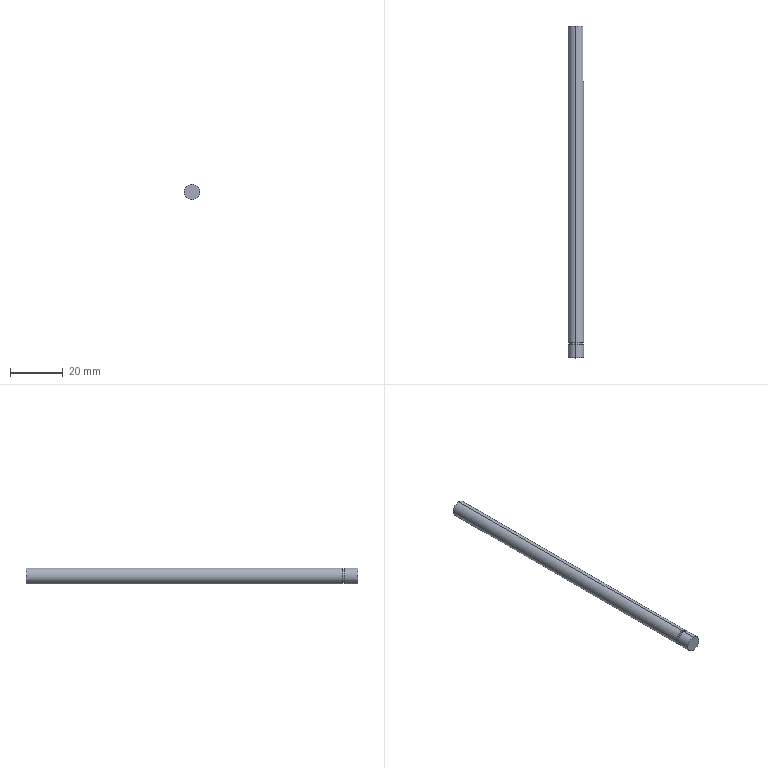Part | STEP file | 1 solid | 12 faces | box 6 x 126 x 6 mm | volume 3530 mm3 | cylinder 6 | plane 6 | commonest cylinder face diameters 6 x4 5 x2
STEP:
#1=CARTESIAN_POINT('',(0.,0.,0.));
#2=DIRECTION('',(0.,0.,1.));
#3=DIRECTION('',(1.,0.,0.));
#4=AXIS2_PLACEMENT_3D('',#1,#2,#3);
#5=CARTESIAN_POINT('',(0.,120.,3.));
#6=VERTEX_POINT('',#5);
#7=CARTESIAN_POINT('',(2.5,120.,1.658));
#8=VERTEX_POINT('',#7);
#9=CARTESIAN_POINT('',(0.,120.,0.));
#10=DIRECTION('',(0.,1.,0.));
#11=DIRECTION('',(0.,0.,1.));
#12=AXIS2_PLACEMENT_3D('',#9,#10,#11);
#13=CIRCLE('',#12,3.);
#14=CARTESIAN_POINT('',(0.,120.,0.));
#15=DIRECTION('',(0.,-1.,0.));
#16=DIRECTION('',(0.,0.,-1.));
#17=AXIS2_PLACEMENT_3D('',#14,#15,#16);
#18=CYLINDRICAL_SURFACE('',#17,3.);
#19=CARTESIAN_POINT('',(3.142,0.));
#20=DIRECTION('',(-1.,0.));
#21=VECTOR('',#20,1.);
#22=LINE('',#19,#21);
#23=(GEOMETRIC_REPRESENTATION_CONTEXT(2)PARAMETRIC_REPRESENTATION_CONTEXT()REPRESENTATION_CONTEXT('',''));
#24=DEFINITIONAL_REPRESENTATION('',(#22),#23);
#25=PCURVE('',#18,#24);
#26=CARTESIAN_POINT('',(0.,120.,0.));
#27=DIRECTION('',(0.,1.,0.));
#28=DIRECTION('',(0.,0.,1.));
#29=AXIS2_PLACEMENT_3D('',#26,#27,#28);
#30=PLANE('',#29);
#31=CARTESIAN_POINT('',(0.,0.));
#32=DIRECTION('',(1.,0.));
#33=AXIS2_PLACEMENT_2D('',#31,#32);
#34=CIRCLE('',#33,3.);
#35=(GEOMETRIC_REPRESENTATION_CONTEXT(2)PARAMETRIC_REPRESENTATION_CONTEXT()REPRESENTATION_CONTEXT('',''));
#36=DEFINITIONAL_REPRESENTATION('',(#34),#35);
#37=PCURVE('',#30,#36);
#38=SURFACE_CURVE('',#13,(#25,#37),.PCURVE_S1.);
#39=EDGE_CURVE('',#6,#8,#38,.T.);
#40=ORIENTED_EDGE('',*,*,#39,.F.);
#41=CARTESIAN_POINT('',(0.,0.,3.));
#42=VERTEX_POINT('',#41);
#43=CARTESIAN_POINT('',(0.,120.,3.));
#44=DIRECTION('',(0.,-1.,0.));
#45=VECTOR('',#44,1.);
#46=LINE('',#43,#45);
#47=CARTESIAN_POINT('',(3.142,0.));
#48=DIRECTION('',(0.,1.));
#49=VECTOR('',#48,1.);
#50=LINE('',#47,#49);
#51=(GEOMETRIC_REPRESENTATION_CONTEXT(2)PARAMETRIC_REPRESENTATION_CONTEXT()REPRESENTATION_CONTEXT('',''));
#52=DEFINITIONAL_REPRESENTATION('',(#50),#51);
#53=PCURVE('',#18,#52);
#54=CARTESIAN_POINT('',(0.,120.,0.));
#55=DIRECTION('',(0.,-1.,0.));
#56=DIRECTION('',(0.,0.,-1.));
#57=AXIS2_PLACEMENT_3D('',#54,#55,#56);
#58=CYLINDRICAL_SURFACE('',#57,3.);
#59=CARTESIAN_POINT('',(3.142,0.));
#60=DIRECTION('',(0.,1.));
#61=VECTOR('',#60,1.);
#62=LINE('',#59,#61);
#63=(GEOMETRIC_REPRESENTATION_CONTEXT(2)PARAMETRIC_REPRESENTATION_CONTEXT()REPRESENTATION_CONTEXT('',''));
#64=DEFINITIONAL_REPRESENTATION('',(#62),#63);
#65=PCURVE('',#58,#64);
#66=SURFACE_CURVE('',#46,(#53,#65),.PCURVE_S1.);
#67=EDGE_CURVE('',#6,#42,#66,.T.);
#68=ORIENTED_EDGE('',*,*,#67,.T.);
#69=CARTESIAN_POINT('',(0.,0.,-3.));
#70=VERTEX_POINT('',#69);
#71=CARTESIAN_POINT('',(0.,0.,0.));
#72=DIRECTION('',(0.,-1.,0.));
#73=DIRECTION('',(0.,0.,-1.));
#74=AXIS2_PLACEMENT_3D('',#71,#72,#73);
#75=CIRCLE('',#74,3.);
#76=CARTESIAN_POINT('',(0.,120.));
#77=DIRECTION('',(1.,0.));
#78=VECTOR('',#77,1.);
#79=LINE('',#76,#78);
#80=(GEOMETRIC_REPRESENTATION_CONTEXT(2)PARAMETRIC_REPRESENTATION_CONTEXT()REPRESENTATION_CONTEXT('',''));
#81=DEFINITIONAL_REPRESENTATION('',(#79),#80);
#82=PCURVE('',#18,#81);
#83=CARTESIAN_POINT('',(0.,0.,0.));
#84=DIRECTION('',(0.,-1.,0.));
#85=DIRECTION('',(0.,0.,-1.));
#86=AXIS2_PLACEMENT_3D('',#83,#84,#85);
#87=PLANE('',#86);
#88=CARTESIAN_POINT('',(0.,0.));
#89=DIRECTION('',(1.,0.));
#90=AXIS2_PLACEMENT_2D('',#88,#89);
#91=CIRCLE('',#90,3.);
#92=(GEOMETRIC_REPRESENTATION_CONTEXT(2)PARAMETRIC_REPRESENTATION_CONTEXT()REPRESENTATION_CONTEXT('',''));
#93=DEFINITIONAL_REPRESENTATION('',(#91),#92);
#94=PCURVE('',#87,#93);
#95=SURFACE_CURVE('',#75,(#82,#94),.PCURVE_S1.);
#96=EDGE_CURVE('',#70,#42,#95,.T.);
#97=ORIENTED_EDGE('',*,*,#96,.F.);
#98=CARTESIAN_POINT('',(0.,120.,-3.));
#99=VERTEX_POINT('',#98);
#100=CARTESIAN_POINT('',(0.,120.,-3.));
#101=DIRECTION('',(0.,-1.,0.));
#102=VECTOR('',#101,1.);
#103=LINE('',#100,#102);
#104=CARTESIAN_POINT('',(0.,0.));
#105=DIRECTION('',(0.,1.));
#106=VECTOR('',#105,1.);
#107=LINE('',#104,#106);
#108=(GEOMETRIC_REPRESENTATION_CONTEXT(2)PARAMETRIC_REPRESENTATION_CONTEXT()REPRESENTATION_CONTEXT('',''));
#109=DEFINITIONAL_REPRESENTATION('',(#107),#108);
#110=PCURVE('',#18,#109);
#111=CARTESIAN_POINT('',(6.283,0.));
#112=DIRECTION('',(0.,1.));
#113=VECTOR('',#112,1.);
#114=LINE('',#111,#113);
#115=(GEOMETRIC_REPRESENTATION_CONTEXT(2)PARAMETRIC_REPRESENTATION_CONTEXT()REPRESENTATION_CONTEXT('',''));
#116=DEFINITIONAL_REPRESENTATION('',(#114),#115);
#117=PCURVE('',#58,#116);
#118=SURFACE_CURVE('',#103,(#110,#117),.PCURVE_S1.);
#119=EDGE_CURVE('',#99,#70,#118,.T.);
#120=ORIENTED_EDGE('',*,*,#119,.F.);
#121=CARTESIAN_POINT('',(2.5,120.,-1.658));
#122=VERTEX_POINT('',#121);
#123=CARTESIAN_POINT('',(0.,120.,0.));
#124=DIRECTION('',(0.,1.,0.));
#125=DIRECTION('',(0.,0.,1.));
#126=AXIS2_PLACEMENT_3D('',#123,#124,#125);
#127=CIRCLE('',#126,3.);
#128=CARTESIAN_POINT('',(3.142,0.));
#129=DIRECTION('',(-1.,0.));
#130=VECTOR('',#129,1.);
#131=LINE('',#128,#130);
#132=(GEOMETRIC_REPRESENTATION_CONTEXT(2)PARAMETRIC_REPRESENTATION_CONTEXT()REPRESENTATION_CONTEXT('',''));
#133=DEFINITIONAL_REPRESENTATION('',(#131),#132);
#134=PCURVE('',#18,#133);
#135=CARTESIAN_POINT('',(0.,0.));
#136=DIRECTION('',(1.,0.));
#137=AXIS2_PLACEMENT_2D('',#135,#136);
#138=CIRCLE('',#137,3.);
#139=(GEOMETRIC_REPRESENTATION_CONTEXT(2)PARAMETRIC_REPRESENTATION_CONTEXT()REPRESENTATION_CONTEXT('',''));
#140=DEFINITIONAL_REPRESENTATION('',(#138),#139);
#141=PCURVE('',#30,#140);
#142=SURFACE_CURVE('',#127,(#134,#141),.PCURVE_S1.);
#143=EDGE_CURVE('',#122,#99,#142,.T.);
#144=ORIENTED_EDGE('',*,*,#143,.F.);
#145=CARTESIAN_POINT('',(2.5,99.,-1.658));
#146=VERTEX_POINT('',#145);
#147=CARTESIAN_POINT('',(2.5,120.,-1.658));
#148=DIRECTION('',(0.,-1.,0.));
#149=VECTOR('',#148,1.);
#150=LINE('',#147,#149);
#151=CARTESIAN_POINT('',(0.9851,0.));
#152=DIRECTION('',(0.,1.));
#153=VECTOR('',#152,1.);
#154=LINE('',#151,#153);
#155=(GEOMETRIC_REPRESENTATION_CONTEXT(2)PARAMETRIC_REPRESENTATION_CONTEXT()REPRESENTATION_CONTEXT('',''));
#156=DEFINITIONAL_REPRESENTATION('',(#154),#155);
#157=PCURVE('',#18,#156);
#158=CARTESIAN_POINT('',(2.5,120.,-3.));
#159=DIRECTION('',(-1.,0.,0.));
#160=DIRECTION('',(0.,-1.,0.));
#161=AXIS2_PLACEMENT_3D('',#158,#159,#160);
#162=PLANE('',#161);
#163=CARTESIAN_POINT('',(0.,1.342));
#164=DIRECTION('',(1.,0.));
#165=VECTOR('',#164,1.);
#166=LINE('',#163,#165);
#167=(GEOMETRIC_REPRESENTATION_CONTEXT(2)PARAMETRIC_REPRESENTATION_CONTEXT()REPRESENTATION_CONTEXT('',''));
#168=DEFINITIONAL_REPRESENTATION('',(#166),#167);
#169=PCURVE('',#162,#168);
#170=SURFACE_CURVE('',#150,(#157,#169),.PCURVE_S1.);
#171=EDGE_CURVE('',#122,#146,#170,.T.);
#172=ORIENTED_EDGE('',*,*,#171,.T.);
#173=CARTESIAN_POINT('',(2.5,99.,1.658));
#174=VERTEX_POINT('',#173);
#175=CARTESIAN_POINT('',(0.,99.,0.));
#176=DIRECTION('',(0.,-1.,0.));
#177=DIRECTION('',(0.,0.,-1.));
#178=AXIS2_PLACEMENT_3D('',#175,#176,#177);
#179=CIRCLE('',#178,3.);
#180=CARTESIAN_POINT('',(0.,21.));
#181=DIRECTION('',(1.,0.));
#182=VECTOR('',#181,1.);
#183=LINE('',#180,#182);
#184=(GEOMETRIC_REPRESENTATION_CONTEXT(2)PARAMETRIC_REPRESENTATION_CONTEXT()REPRESENTATION_CONTEXT('',''));
#185=DEFINITIONAL_REPRESENTATION('',(#183),#184);
#186=PCURVE('',#18,#185);
#187=CARTESIAN_POINT('',(3.,99.,-3.));
#188=DIRECTION('',(0.,-1.,0.));
#189=DIRECTION('',(0.,0.,-1.));
#190=AXIS2_PLACEMENT_3D('',#187,#188,#189);
#191=PLANE('',#190);
#192=CARTESIAN_POINT('',(-3.,-3.));
#193=DIRECTION('',(1.,0.));
#194=AXIS2_PLACEMENT_2D('',#192,#193);
#195=CIRCLE('',#194,3.);
#196=(GEOMETRIC_REPRESENTATION_CONTEXT(2)PARAMETRIC_REPRESENTATION_CONTEXT()REPRESENTATION_CONTEXT('',''));
#197=DEFINITIONAL_REPRESENTATION('',(#195),#196);
#198=PCURVE('',#191,#197);
#199=SURFACE_CURVE('',#179,(#186,#198),.PCURVE_S1.);
#200=EDGE_CURVE('',#146,#174,#199,.T.);
#201=ORIENTED_EDGE('',*,*,#200,.T.);
#202=CARTESIAN_POINT('',(2.5,120.,1.658));
#203=DIRECTION('',(0.,1.,0.));
#204=VECTOR('',#203,1.);
#205=LINE('',#202,#204);
#206=CARTESIAN_POINT('',(2.156,0.));
#207=DIRECTION('',(0.,-1.));
#208=VECTOR('',#207,1.);
#209=LINE('',#206,#208);
#210=(GEOMETRIC_REPRESENTATION_CONTEXT(2)PARAMETRIC_REPRESENTATION_CONTEXT()REPRESENTATION_CONTEXT('',''));
#211=DEFINITIONAL_REPRESENTATION('',(#209),#210);
#212=PCURVE('',#18,#211);
#213=CARTESIAN_POINT('',(0.,4.658));
#214=DIRECTION('',(-1.,0.));
#215=VECTOR('',#214,1.);
#216=LINE('',#213,#215);
#217=(GEOMETRIC_REPRESENTATION_CONTEXT(2)PARAMETRIC_REPRESENTATION_CONTEXT()REPRESENTATION_CONTEXT('',''));
#218=DEFINITIONAL_REPRESENTATION('',(#216),#217);
#219=PCURVE('',#162,#218);
#220=SURFACE_CURVE('',#205,(#212,#219),.PCURVE_S1.);
#221=EDGE_CURVE('',#174,#8,#220,.T.);
#222=ORIENTED_EDGE('',*,*,#221,.T.);
#223=EDGE_LOOP('',(#40,#68,#97,#120,#144,#172,#201,#222));
#224=FACE_BOUND('',#223,.T.);
#225=ADVANCED_FACE('',(#224),#18,.T.);
#226=CARTESIAN_POINT('',(0.,-1.,-2.5));
#227=VERTEX_POINT('',#226);
#228=CARTESIAN_POINT('',(0.,-1.,2.5));
#229=VERTEX_POINT('',#228);
#230=CARTESIAN_POINT('',(0.,-1.,0.));
#231=DIRECTION('',(0.,-1.,0.));
#232=DIRECTION('',(0.,0.,-1.));
#233=AXIS2_PLACEMENT_3D('',#230,#231,#232);
#234=CIRCLE('',#233,2.5);
#235=CARTESIAN_POINT('',(0.,-1.,0.));
#236=DIRECTION('',(0.,1.,0.));
#237=DIRECTION('',(0.,0.,1.));
#238=AXIS2_PLACEMENT_3D('',#235,#236,#237);
#239=CYLINDRICAL_SURFACE('',#238,2.5);
#240=CARTESIAN_POINT('',(3.142,0.));
#241=DIRECTION('',(-1.,0.));
#242=VECTOR('',#241,1.);
#243=LINE('',#240,#242);
#244=(GEOMETRIC_REPRESENTATION_CONTEXT(2)PARAMETRIC_REPRESENTATION_CONTEXT()REPRESENTATION_CONTEXT('',''));
#245=DEFINITIONAL_REPRESENTATION('',(#243),#244);
#246=PCURVE('',#239,#245);
#247=CARTESIAN_POINT('',(0.,-1.,0.));
#248=DIRECTION('',(0.,-1.,0.));
#249=DIRECTION('',(0.,0.,-1.));
#250=AXIS2_PLACEMENT_3D('',#247,#248,#249);
#251=PLANE('',#250);
#252=CARTESIAN_POINT('',(0.,0.));
#253=DIRECTION('',(1.,0.));
#254=AXIS2_PLACEMENT_2D('',#252,#253);
#255=CIRCLE('',#254,2.5);
#256=(GEOMETRIC_REPRESENTATION_CONTEXT(2)PARAMETRIC_REPRESENTATION_CONTEXT()REPRESENTATION_CONTEXT('',''));
#257=DEFINITIONAL_REPRESENTATION('',(#255),#256);
#258=PCURVE('',#251,#257);
#259=SURFACE_CURVE('',#234,(#246,#258),.PCURVE_S1.);
#260=EDGE_CURVE('',#227,#229,#259,.T.);
#261=ORIENTED_EDGE('',*,*,#260,.F.);
#262=CARTESIAN_POINT('',(0.,0.,-2.5));
#263=VERTEX_POINT('',#262);
#264=CARTESIAN_POINT('',(0.,-1.,-2.5));
#265=DIRECTION('',(0.,1.,0.));
#266=VECTOR('',#265,1.);
#267=LINE('',#264,#266);
#268=CARTESIAN_POINT('',(3.142,0.));
#269=DIRECTION('',(0.,1.));
#270=VECTOR('',#269,1.);
#271=LINE('',#268,#270);
#272=(GEOMETRIC_REPRESENTATION_CONTEXT(2)PARAMETRIC_REPRESENTATION_CONTEXT()REPRESENTATION_CONTEXT('',''));
#273=DEFINITIONAL_REPRESENTATION('',(#271),#272);
#274=PCURVE('',#239,#273);
#275=CARTESIAN_POINT('',(0.,-1.,0.));
#276=DIRECTION('',(0.,1.,0.));
#277=DIRECTION('',(0.,0.,1.));
#278=AXIS2_PLACEMENT_3D('',#275,#276,#277);
#279=CYLINDRICAL_SURFACE('',#278,2.5);
#280=CARTESIAN_POINT('',(3.142,0.));
#281=DIRECTION('',(0.,1.));
#282=VECTOR('',#281,1.);
#283=LINE('',#280,#282);
#284=(GEOMETRIC_REPRESENTATION_CONTEXT(2)PARAMETRIC_REPRESENTATION_CONTEXT()REPRESENTATION_CONTEXT('',''));
#285=DEFINITIONAL_REPRESENTATION('',(#283),#284);
#286=PCURVE('',#279,#285);
#287=SURFACE_CURVE('',#267,(#274,#286),.PCURVE_S1.);
#288=EDGE_CURVE('',#227,#263,#287,.T.);
#289=ORIENTED_EDGE('',*,*,#288,.T.);
#290=CARTESIAN_POINT('',(0.,0.,2.5));
#291=VERTEX_POINT('',#290);
#292=CARTESIAN_POINT('',(0.,0.,0.));
#293=DIRECTION('',(0.,-1.,0.));
#294=DIRECTION('',(0.,0.,-1.));
#295=AXIS2_PLACEMENT_3D('',#292,#293,#294);
#296=CIRCLE('',#295,2.5);
#297=CARTESIAN_POINT('',(3.142,1.));
#298=DIRECTION('',(-1.,0.));
#299=VECTOR('',#298,1.);
#300=LINE('',#297,#299);
#301=(GEOMETRIC_REPRESENTATION_CONTEXT(2)PARAMETRIC_REPRESENTATION_CONTEXT()REPRESENTATION_CONTEXT('',''));
#302=DEFINITIONAL_REPRESENTATION('',(#300),#301);
#303=PCURVE('',#239,#302);
#304=CARTESIAN_POINT('',(0.,0.));
#305=DIRECTION('',(1.,0.));
#306=AXIS2_PLACEMENT_2D('',#304,#305);
#307=CIRCLE('',#306,2.5);
#308=(GEOMETRIC_REPRESENTATION_CONTEXT(2)PARAMETRIC_REPRESENTATION_CONTEXT()REPRESENTATION_CONTEXT('',''));
#309=DEFINITIONAL_REPRESENTATION('',(#307),#308);
#310=PCURVE('',#87,#309);
#311=SURFACE_CURVE('',#296,(#303,#310),.PCURVE_S1.);
#312=EDGE_CURVE('',#263,#291,#311,.T.);
#313=ORIENTED_EDGE('',*,*,#312,.T.);
#314=CARTESIAN_POINT('',(0.,-1.,2.5));
#315=DIRECTION('',(0.,1.,0.));
#316=VECTOR('',#315,1.);
#317=LINE('',#314,#316);
#318=CARTESIAN_POINT('',(0.,0.));
#319=DIRECTION('',(0.,1.));
#320=VECTOR('',#319,1.);
#321=LINE('',#318,#320);
#322=(GEOMETRIC_REPRESENTATION_CONTEXT(2)PARAMETRIC_REPRESENTATION_CONTEXT()REPRESENTATION_CONTEXT('',''));
#323=DEFINITIONAL_REPRESENTATION('',(#321),#322);
#324=PCURVE('',#239,#323);
#325=CARTESIAN_POINT('',(6.283,0.));
#326=DIRECTION('',(0.,1.));
#327=VECTOR('',#326,1.);
#328=LINE('',#325,#327);
#329=(GEOMETRIC_REPRESENTATION_CONTEXT(2)PARAMETRIC_REPRESENTATION_CONTEXT()REPRESENTATION_CONTEXT('',''));
#330=DEFINITIONAL_REPRESENTATION('',(#328),#329);
#331=PCURVE('',#279,#330);
#332=SURFACE_CURVE('',#317,(#324,#331),.PCURVE_S1.);
#333=EDGE_CURVE('',#229,#291,#332,.T.);
#334=ORIENTED_EDGE('',*,*,#333,.F.);
#335=EDGE_LOOP('',(#261,#289,#313,#334));
#336=FACE_BOUND('',#335,.T.);
#337=ADVANCED_FACE('',(#336),#239,.T.);
#338=CARTESIAN_POINT('',(0.,-1.,-3.));
#339=VERTEX_POINT('',#338);
#340=CARTESIAN_POINT('',(0.,-1.,3.));
#341=VERTEX_POINT('',#340);
#342=CARTESIAN_POINT('',(0.,-1.,0.));
#343=DIRECTION('',(0.,-1.,0.));
#344=DIRECTION('',(0.,0.,-1.));
#345=AXIS2_PLACEMENT_3D('',#342,#343,#344);
#346=CIRCLE('',#345,3.);
#347=CARTESIAN_POINT('',(0.,120.,0.));
#348=DIRECTION('',(0.,-1.,0.));
#349=DIRECTION('',(0.,0.,-1.));
#350=AXIS2_PLACEMENT_3D('',#347,#348,#349);
#351=CYLINDRICAL_SURFACE('',#350,3.);
#352=CARTESIAN_POINT('',(0.,121.));
#353=DIRECTION('',(1.,0.));
#354=VECTOR('',#353,1.);
#355=LINE('',#352,#354);
#356=(GEOMETRIC_REPRESENTATION_CONTEXT(2)PARAMETRIC_REPRESENTATION_CONTEXT()REPRESENTATION_CONTEXT('',''));
#357=DEFINITIONAL_REPRESENTATION('',(#355),#356);
#358=PCURVE('',#351,#357);
#359=CARTESIAN_POINT('',(0.,0.));
#360=DIRECTION('',(1.,0.));
#361=AXIS2_PLACEMENT_2D('',#359,#360);
#362=CIRCLE('',#361,3.);
#363=(GEOMETRIC_REPRESENTATION_CONTEXT(2)PARAMETRIC_REPRESENTATION_CONTEXT()REPRESENTATION_CONTEXT('',''));
#364=DEFINITIONAL_REPRESENTATION('',(#362),#363);
#365=PCURVE('',#251,#364);
#366=SURFACE_CURVE('',#346,(#358,#365),.PCURVE_S1.);
#367=EDGE_CURVE('',#339,#341,#366,.T.);
#368=ORIENTED_EDGE('',*,*,#367,.T.);
#369=CARTESIAN_POINT('',(0.,-6.,3.));
#370=VERTEX_POINT('',#369);
#371=CARTESIAN_POINT('',(0.,120.,3.));
#372=DIRECTION('',(0.,-1.,0.));
#373=VECTOR('',#372,1.);
#374=LINE('',#371,#373);
#375=CARTESIAN_POINT('',(3.142,0.));
#376=DIRECTION('',(0.,1.));
#377=VECTOR('',#376,1.);
#378=LINE('',#375,#377);
#379=(GEOMETRIC_REPRESENTATION_CONTEXT(2)PARAMETRIC_REPRESENTATION_CONTEXT()REPRESENTATION_CONTEXT('',''));
#380=DEFINITIONAL_REPRESENTATION('',(#378),#379);
#381=PCURVE('',#351,#380);
#382=CARTESIAN_POINT('',(0.,120.,0.));
#383=DIRECTION('',(0.,-1.,0.));
#384=DIRECTION('',(0.,0.,-1.));
#385=AXIS2_PLACEMENT_3D('',#382,#383,#384);
#386=CYLINDRICAL_SURFACE('',#385,3.);
#387=CARTESIAN_POINT('',(3.142,0.));
#388=DIRECTION('',(0.,1.));
#389=VECTOR('',#388,1.);
#390=LINE('',#387,#389);
#391=(GEOMETRIC_REPRESENTATION_CONTEXT(2)PARAMETRIC_REPRESENTATION_CONTEXT()REPRESENTATION_CONTEXT('',''));
#392=DEFINITIONAL_REPRESENTATION('',(#390),#391);
#393=PCURVE('',#386,#392);
#394=SURFACE_CURVE('',#374,(#381,#393),.PCURVE_S1.);
#395=EDGE_CURVE('',#341,#370,#394,.T.);
#396=ORIENTED_EDGE('',*,*,#395,.T.);
#397=CARTESIAN_POINT('',(0.,-6.,-3.));
#398=VERTEX_POINT('',#397);
#399=CARTESIAN_POINT('',(0.,-6.,0.));
#400=DIRECTION('',(0.,-1.,0.));
#401=DIRECTION('',(0.,0.,-1.));
#402=AXIS2_PLACEMENT_3D('',#399,#400,#401);
#403=CIRCLE('',#402,3.);
#404=CARTESIAN_POINT('',(0.,126.));
#405=DIRECTION('',(1.,0.));
#406=VECTOR('',#405,1.);
#407=LINE('',#404,#406);
#408=(GEOMETRIC_REPRESENTATION_CONTEXT(2)PARAMETRIC_REPRESENTATION_CONTEXT()REPRESENTATION_CONTEXT('',''));
#409=DEFINITIONAL_REPRESENTATION('',(#407),#408);
#410=PCURVE('',#351,#409);
#411=CARTESIAN_POINT('',(0.,-6.,0.));
#412=DIRECTION('',(0.,-1.,0.));
#413=DIRECTION('',(0.,0.,-1.));
#414=AXIS2_PLACEMENT_3D('',#411,#412,#413);
#415=PLANE('',#414);
#416=CARTESIAN_POINT('',(0.,0.));
#417=DIRECTION('',(1.,0.));
#418=AXIS2_PLACEMENT_2D('',#416,#417);
#419=CIRCLE('',#418,3.);
#420=(GEOMETRIC_REPRESENTATION_CONTEXT(2)PARAMETRIC_REPRESENTATION_CONTEXT()REPRESENTATION_CONTEXT('',''));
#421=DEFINITIONAL_REPRESENTATION('',(#419),#420);
#422=PCURVE('',#415,#421);
#423=SURFACE_CURVE('',#403,(#410,#422),.PCURVE_S1.);
#424=EDGE_CURVE('',#398,#370,#423,.T.);
#425=ORIENTED_EDGE('',*,*,#424,.F.);
#426=CARTESIAN_POINT('',(0.,120.,-3.));
#427=DIRECTION('',(0.,-1.,0.));
#428=VECTOR('',#427,1.);
#429=LINE('',#426,#428);
#430=CARTESIAN_POINT('',(0.,0.));
#431=DIRECTION('',(0.,1.));
#432=VECTOR('',#431,1.);
#433=LINE('',#430,#432);
#434=(GEOMETRIC_REPRESENTATION_CONTEXT(2)PARAMETRIC_REPRESENTATION_CONTEXT()REPRESENTATION_CONTEXT('',''));
#435=DEFINITIONAL_REPRESENTATION('',(#433),#434);
#436=PCURVE('',#351,#435);
#437=CARTESIAN_POINT('',(6.283,0.));
#438=DIRECTION('',(0.,1.));
#439=VECTOR('',#438,1.);
#440=LINE('',#437,#439);
#441=(GEOMETRIC_REPRESENTATION_CONTEXT(2)PARAMETRIC_REPRESENTATION_CONTEXT()REPRESENTATION_CONTEXT('',''));
#442=DEFINITIONAL_REPRESENTATION('',(#440),#441);
#443=PCURVE('',#386,#442);
#444=SURFACE_CURVE('',#429,(#436,#443),.PCURVE_S1.);
#445=EDGE_CURVE('',#339,#398,#444,.T.);
#446=ORIENTED_EDGE('',*,*,#445,.F.);
#447=EDGE_LOOP('',(#368,#396,#425,#446));
#448=FACE_BOUND('',#447,.T.);
#449=ADVANCED_FACE('',(#448),#351,.T.);
#450=ORIENTED_EDGE('',*,*,#395,.F.);
#451=CARTESIAN_POINT('',(0.,-1.,0.));
#452=DIRECTION('',(0.,-1.,0.));
#453=DIRECTION('',(0.,0.,-1.));
#454=AXIS2_PLACEMENT_3D('',#451,#452,#453);
#455=CIRCLE('',#454,3.);
#456=CARTESIAN_POINT('',(0.,121.));
#457=DIRECTION('',(1.,0.));
#458=VECTOR('',#457,1.);
#459=LINE('',#456,#458);
#460=(GEOMETRIC_REPRESENTATION_CONTEXT(2)PARAMETRIC_REPRESENTATION_CONTEXT()REPRESENTATION_CONTEXT('',''));
#461=DEFINITIONAL_REPRESENTATION('',(#459),#460);
#462=PCURVE('',#386,#461);
#463=CARTESIAN_POINT('',(0.,0.));
#464=DIRECTION('',(1.,0.));
#465=AXIS2_PLACEMENT_2D('',#463,#464);
#466=CIRCLE('',#465,3.);
#467=(GEOMETRIC_REPRESENTATION_CONTEXT(2)PARAMETRIC_REPRESENTATION_CONTEXT()REPRESENTATION_CONTEXT('',''));
#468=DEFINITIONAL_REPRESENTATION('',(#466),#467);
#469=PCURVE('',#251,#468);
#470=SURFACE_CURVE('',#455,(#462,#469),.PCURVE_S1.);
#471=EDGE_CURVE('',#341,#339,#470,.T.);
#472=ORIENTED_EDGE('',*,*,#471,.T.);
#473=ORIENTED_EDGE('',*,*,#445,.T.);
#474=CARTESIAN_POINT('',(0.,-6.,0.));
#475=DIRECTION('',(0.,-1.,0.));
#476=DIRECTION('',(0.,0.,-1.));
#477=AXIS2_PLACEMENT_3D('',#474,#475,#476);
#478=CIRCLE('',#477,3.);
#479=CARTESIAN_POINT('',(0.,126.));
#480=DIRECTION('',(1.,0.));
#481=VECTOR('',#480,1.);
#482=LINE('',#479,#481);
#483=(GEOMETRIC_REPRESENTATION_CONTEXT(2)PARAMETRIC_REPRESENTATION_CONTEXT()REPRESENTATION_CONTEXT('',''));
#484=DEFINITIONAL_REPRESENTATION('',(#482),#483);
#485=PCURVE('',#386,#484);
#486=CARTESIAN_POINT('',(0.,0.));
#487=DIRECTION('',(1.,0.));
#488=AXIS2_PLACEMENT_2D('',#486,#487);
#489=CIRCLE('',#488,3.);
#490=(GEOMETRIC_REPRESENTATION_CONTEXT(2)PARAMETRIC_REPRESENTATION_CONTEXT()REPRESENTATION_CONTEXT('',''));
#491=DEFINITIONAL_REPRESENTATION('',(#489),#490);
#492=PCURVE('',#415,#491);
#493=SURFACE_CURVE('',#478,(#485,#492),.PCURVE_S1.);
#494=EDGE_CURVE('',#370,#398,#493,.T.);
#495=ORIENTED_EDGE('',*,*,#494,.F.);
#496=EDGE_LOOP('',(#450,#472,#473,#495));
#497=FACE_BOUND('',#496,.T.);
#498=ADVANCED_FACE('',(#497),#386,.T.);
#499=ORIENTED_EDGE('',*,*,#424,.T.);
#500=ORIENTED_EDGE('',*,*,#494,.T.);
#501=EDGE_LOOP('',(#499,#500));
#502=FACE_BOUND('',#501,.T.);
#503=ADVANCED_FACE('',(#502),#415,.T.);
#504=ORIENTED_EDGE('',*,*,#367,.F.);
#505=ORIENTED_EDGE('',*,*,#471,.F.);
#506=EDGE_LOOP('',(#504,#505));
#507=FACE_BOUND('',#506,.T.);
#508=CARTESIAN_POINT('',(0.,-1.,0.));
#509=DIRECTION('',(0.,-1.,0.));
#510=DIRECTION('',(0.,0.,-1.));
#511=AXIS2_PLACEMENT_3D('',#508,#509,#510);
#512=CIRCLE('',#511,2.5);
#513=CARTESIAN_POINT('',(0.,0.));
#514=DIRECTION('',(1.,0.));
#515=AXIS2_PLACEMENT_2D('',#513,#514);
#516=CIRCLE('',#515,2.5);
#517=(GEOMETRIC_REPRESENTATION_CONTEXT(2)PARAMETRIC_REPRESENTATION_CONTEXT()REPRESENTATION_CONTEXT('',''));
#518=DEFINITIONAL_REPRESENTATION('',(#516),#517);
#519=PCURVE('',#251,#518);
#520=CARTESIAN_POINT('',(9.425,0.));
#521=DIRECTION('',(-1.,0.));
#522=VECTOR('',#521,1.);
#523=LINE('',#520,#522);
#524=(GEOMETRIC_REPRESENTATION_CONTEXT(2)PARAMETRIC_REPRESENTATION_CONTEXT()REPRESENTATION_CONTEXT('',''));
#525=DEFINITIONAL_REPRESENTATION('',(#523),#524);
#526=PCURVE('',#279,#525);
#527=SURFACE_CURVE('',#512,(#519,#526),.PCURVE_S1.);
#528=EDGE_CURVE('',#229,#227,#527,.T.);
#529=ORIENTED_EDGE('',*,*,#528,.T.);
#530=ORIENTED_EDGE('',*,*,#260,.T.);
#531=EDGE_LOOP('',(#529,#530));
#532=FACE_BOUND('',#531,.T.);
#533=ADVANCED_FACE('',(#507,#532),#251,.F.);
#534=ORIENTED_EDGE('',*,*,#96,.T.);
#535=CARTESIAN_POINT('',(0.,0.,0.));
#536=DIRECTION('',(0.,-1.,0.));
#537=DIRECTION('',(0.,0.,-1.));
#538=AXIS2_PLACEMENT_3D('',#535,#536,#537);
#539=CIRCLE('',#538,3.);
#540=CARTESIAN_POINT('',(0.,0.));
#541=DIRECTION('',(1.,0.));
#542=AXIS2_PLACEMENT_2D('',#540,#541);
#543=CIRCLE('',#542,3.);
#544=(GEOMETRIC_REPRESENTATION_CONTEXT(2)PARAMETRIC_REPRESENTATION_CONTEXT()REPRESENTATION_CONTEXT('',''));
#545=DEFINITIONAL_REPRESENTATION('',(#543),#544);
#546=PCURVE('',#87,#545);
#547=CARTESIAN_POINT('',(0.,120.));
#548=DIRECTION('',(1.,0.));
#549=VECTOR('',#548,1.);
#550=LINE('',#547,#549);
#551=(GEOMETRIC_REPRESENTATION_CONTEXT(2)PARAMETRIC_REPRESENTATION_CONTEXT()REPRESENTATION_CONTEXT('',''));
#552=DEFINITIONAL_REPRESENTATION('',(#550),#551);
#553=PCURVE('',#58,#552);
#554=SURFACE_CURVE('',#539,(#546,#553),.PCURVE_S1.);
#555=EDGE_CURVE('',#42,#70,#554,.T.);
#556=ORIENTED_EDGE('',*,*,#555,.T.);
#557=EDGE_LOOP('',(#534,#556));
#558=FACE_BOUND('',#557,.T.);
#559=CARTESIAN_POINT('',(0.,0.,0.));
#560=DIRECTION('',(0.,-1.,0.));
#561=DIRECTION('',(0.,0.,-1.));
#562=AXIS2_PLACEMENT_3D('',#559,#560,#561);
#563=CIRCLE('',#562,2.5);
#564=CARTESIAN_POINT('',(0.,0.));
#565=DIRECTION('',(1.,0.));
#566=AXIS2_PLACEMENT_2D('',#564,#565);
#567=CIRCLE('',#566,2.5);
#568=(GEOMETRIC_REPRESENTATION_CONTEXT(2)PARAMETRIC_REPRESENTATION_CONTEXT()REPRESENTATION_CONTEXT('',''));
#569=DEFINITIONAL_REPRESENTATION('',(#567),#568);
#570=PCURVE('',#87,#569);
#571=CARTESIAN_POINT('',(9.425,1.));
#572=DIRECTION('',(-1.,0.));
#573=VECTOR('',#572,1.);
#574=LINE('',#571,#573);
#575=(GEOMETRIC_REPRESENTATION_CONTEXT(2)PARAMETRIC_REPRESENTATION_CONTEXT()REPRESENTATION_CONTEXT('',''));
#576=DEFINITIONAL_REPRESENTATION('',(#574),#575);
#577=PCURVE('',#279,#576);
#578=SURFACE_CURVE('',#563,(#570,#577),.PCURVE_S1.);
#579=EDGE_CURVE('',#291,#263,#578,.T.);
#580=ORIENTED_EDGE('',*,*,#579,.F.);
#581=ORIENTED_EDGE('',*,*,#312,.F.);
#582=EDGE_LOOP('',(#580,#581));
#583=FACE_BOUND('',#582,.T.);
#584=ADVANCED_FACE('',(#558,#583),#87,.T.);
#585=ORIENTED_EDGE('',*,*,#288,.F.);
#586=ORIENTED_EDGE('',*,*,#528,.F.);
#587=ORIENTED_EDGE('',*,*,#333,.T.);
#588=ORIENTED_EDGE('',*,*,#579,.T.);
#589=EDGE_LOOP('',(#585,#586,#587,#588));
#590=FACE_BOUND('',#589,.T.);
#591=ADVANCED_FACE('',(#590),#279,.T.);
#592=CARTESIAN_POINT('',(2.5,99.,-3.));
#593=DIRECTION('',(0.,0.,1.));
#594=VECTOR('',#593,1.);
#595=LINE('',#592,#594);
#596=CARTESIAN_POINT('',(0.,-0.5));
#597=DIRECTION('',(-1.,0.));
#598=VECTOR('',#597,1.);
#599=LINE('',#596,#598);
#600=(GEOMETRIC_REPRESENTATION_CONTEXT(2)PARAMETRIC_REPRESENTATION_CONTEXT()REPRESENTATION_CONTEXT('',''));
#601=DEFINITIONAL_REPRESENTATION('',(#599),#600);
#602=PCURVE('',#191,#601);
#603=CARTESIAN_POINT('',(21.,0.));
#604=DIRECTION('',(0.,1.));
#605=VECTOR('',#604,1.);
#606=LINE('',#603,#605);
#607=(GEOMETRIC_REPRESENTATION_CONTEXT(2)PARAMETRIC_REPRESENTATION_CONTEXT()REPRESENTATION_CONTEXT('',''));
#608=DEFINITIONAL_REPRESENTATION('',(#606),#607);
#609=PCURVE('',#162,#608);
#610=SURFACE_CURVE('',#595,(#602,#609),.PCURVE_S1.);
#611=EDGE_CURVE('',#146,#174,#610,.T.);
#612=ORIENTED_EDGE('',*,*,#611,.T.);
#613=ORIENTED_EDGE('',*,*,#200,.F.);
#614=EDGE_LOOP('',(#612,#613));
#615=FACE_BOUND('',#614,.T.);
#616=ADVANCED_FACE('',(#615),#191,.F.);
#617=CARTESIAN_POINT('',(2.5,120.,0.));
#618=DIRECTION('',(0.,0.,1.));
#619=VECTOR('',#618,1.);
#620=LINE('',#617,#619);
#621=CARTESIAN_POINT('',(0.,3.));
#622=DIRECTION('',(0.,1.));
#623=VECTOR('',#622,1.);
#624=LINE('',#621,#623);
#625=(GEOMETRIC_REPRESENTATION_CONTEXT(2)PARAMETRIC_REPRESENTATION_CONTEXT()REPRESENTATION_CONTEXT('',''));
#626=DEFINITIONAL_REPRESENTATION('',(#624),#625);
#627=PCURVE('',#162,#626);
#628=CARTESIAN_POINT('',(0.,2.5));
#629=DIRECTION('',(1.,0.));
#630=VECTOR('',#629,1.);
#631=LINE('',#628,#630);
#632=(GEOMETRIC_REPRESENTATION_CONTEXT(2)PARAMETRIC_REPRESENTATION_CONTEXT()REPRESENTATION_CONTEXT('',''));
#633=DEFINITIONAL_REPRESENTATION('',(#631),#632);
#634=PCURVE('',#30,#633);
#635=SURFACE_CURVE('',#620,(#627,#634),.PCURVE_S1.);
#636=EDGE_CURVE('',#122,#8,#635,.T.);
#637=ORIENTED_EDGE('',*,*,#636,.T.);
#638=ORIENTED_EDGE('',*,*,#221,.F.);
#639=ORIENTED_EDGE('',*,*,#611,.F.);
#640=ORIENTED_EDGE('',*,*,#171,.F.);
#641=EDGE_LOOP('',(#637,#638,#639,#640));
#642=FACE_BOUND('',#641,.T.);
#643=ADVANCED_FACE('',(#642),#162,.F.);
#644=ORIENTED_EDGE('',*,*,#636,.F.);
#645=ORIENTED_EDGE('',*,*,#143,.T.);
#646=CARTESIAN_POINT('',(0.,120.,0.));
#647=DIRECTION('',(0.,1.,0.));
#648=DIRECTION('',(0.,0.,1.));
#649=AXIS2_PLACEMENT_3D('',#646,#647,#648);
#650=CIRCLE('',#649,3.);
#651=CARTESIAN_POINT('',(0.,0.));
#652=DIRECTION('',(1.,0.));
#653=AXIS2_PLACEMENT_2D('',#651,#652);
#654=CIRCLE('',#653,3.);
#655=(GEOMETRIC_REPRESENTATION_CONTEXT(2)PARAMETRIC_REPRESENTATION_CONTEXT()REPRESENTATION_CONTEXT('',''));
#656=DEFINITIONAL_REPRESENTATION('',(#654),#655);
#657=PCURVE('',#30,#656);
#658=CARTESIAN_POINT('',(9.425,0.));
#659=DIRECTION('',(-1.,0.));
#660=VECTOR('',#659,1.);
#661=LINE('',#658,#660);
#662=(GEOMETRIC_REPRESENTATION_CONTEXT(2)PARAMETRIC_REPRESENTATION_CONTEXT()REPRESENTATION_CONTEXT('',''));
#663=DEFINITIONAL_REPRESENTATION('',(#661),#662);
#664=PCURVE('',#58,#663);
#665=SURFACE_CURVE('',#650,(#657,#664),.PCURVE_S1.);
#666=EDGE_CURVE('',#99,#6,#665,.T.);
#667=ORIENTED_EDGE('',*,*,#666,.T.);
#668=ORIENTED_EDGE('',*,*,#39,.T.);
#669=EDGE_LOOP('',(#644,#645,#667,#668));
#670=FACE_BOUND('',#669,.T.);
#671=ADVANCED_FACE('',(#670),#30,.T.);
#672=ORIENTED_EDGE('',*,*,#67,.F.);
#673=ORIENTED_EDGE('',*,*,#666,.F.);
#674=ORIENTED_EDGE('',*,*,#119,.T.);
#675=ORIENTED_EDGE('',*,*,#555,.F.);
#676=EDGE_LOOP('',(#672,#673,#674,#675));
#677=FACE_BOUND('',#676,.T.);
#678=ADVANCED_FACE('',(#677),#58,.T.);
#679=CLOSED_SHELL('',(#225,#337,#449,#498,#503,#533,#584,#591,#616,#643,#671,#678));
#680=MANIFOLD_SOLID_BREP('',#679);
#681=(LENGTH_UNIT()NAMED_UNIT(*)SI_UNIT(.MILLI.,.METRE.));
#682=UNCERTAINTY_MEASURE_WITH_UNIT(LENGTH_MEASURE(0.0000001),#681,'','');
#683=(NAMED_UNIT(*)PLANE_ANGLE_UNIT()SI_UNIT($,.RADIAN.));
#684=(NAMED_UNIT(*)SI_UNIT($,.STERADIAN.)SOLID_ANGLE_UNIT());
#685=(GEOMETRIC_REPRESENTATION_CONTEXT(3)GLOBAL_UNCERTAINTY_ASSIGNED_CONTEXT((#682))GLOBAL_UNIT_ASSIGNED_CONTEXT((#681,#683,#684))REPRESENTATION_CONTEXT('',''));
#686=ADVANCED_BREP_SHAPE_REPRESENTATION('',(#4,#680),#685);